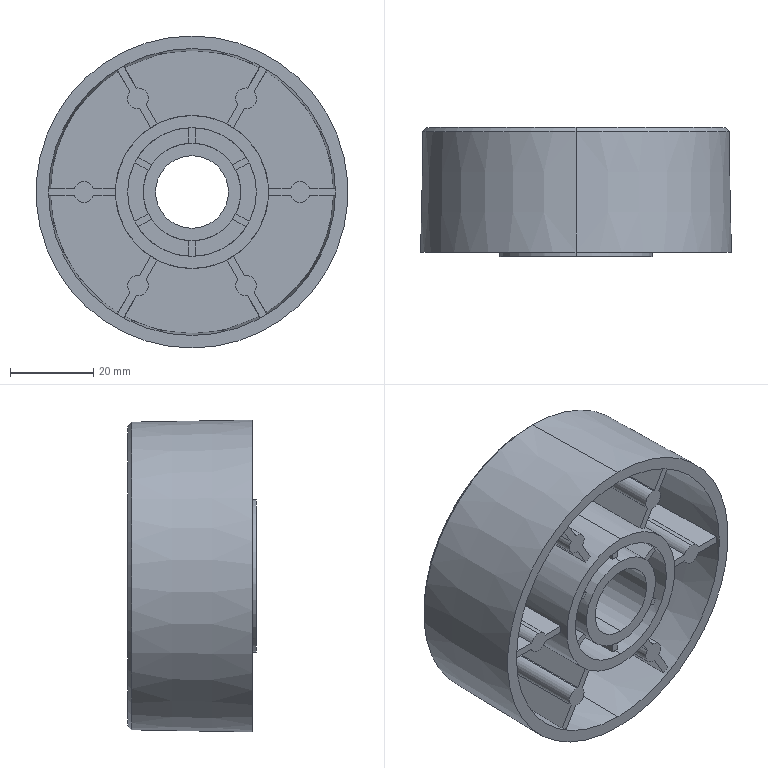Part | SolidWorks | features ICE 14, Rib 6, HoleWzd 2, BaseBody 1, Chamfer 1 | 1 solid | 99 faces | box 75 x 31 x 75 mm | volume 50473 mm3 | plane 65 | cylinder 28 | cone 6 | commonest cylinder face diameters 5 x18 17.5 x2 23.5 x2 30 x2 31 x2 36.8 x2